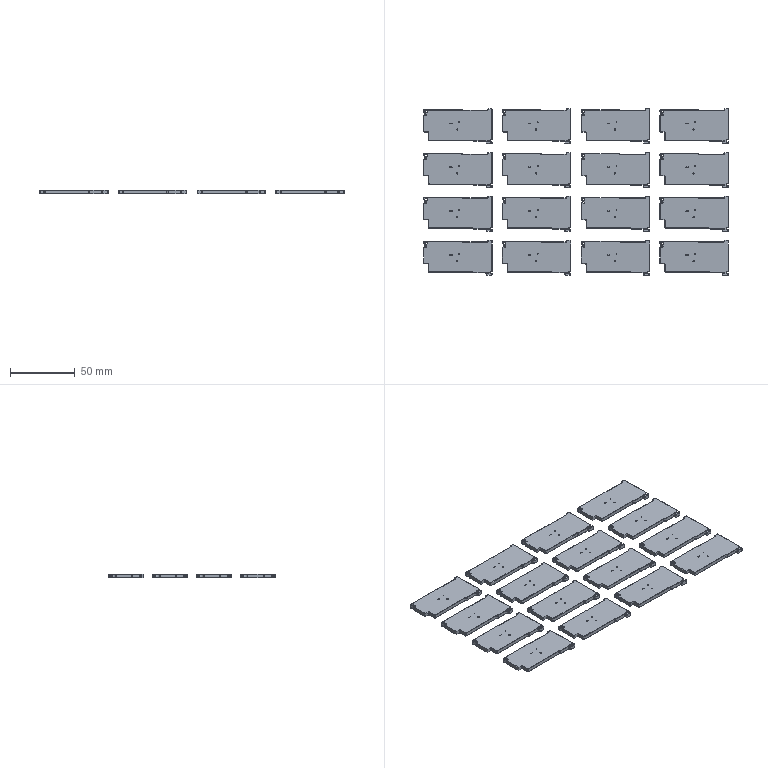NC program | NX | posted with a generic post | part box 236.046 x 129.136 x 3 mm
Whole program:
N10 G17 G21 G94 G90
(DRILLING_COPY , TOOL : D4A45)
N12 T02 M6
N14 G54
N16 G17 G0 G90 X3.25 Y-25.136 S5000 M3
N18 G43 Z30. H2
N20 G94 G81 G98 Z-0.6 F250. R3.
N22 X26.95 Y-16.156
N24 X25.72 Y-10.476
N26 X31.181 Y-11.492
N28 X32.578
N30 X51.15 Y-2.336
N32 X51.058 Y-4.776
N34 G80
N36 G0 X51.058 Y-4.776 Z30.
N38 M5
(DRILLING_COPY_COPY_COPY_COPY_COPY , TOOL : 1.8ZT)
N40 T18 M6
N42 G54
N44 G17 G0 G90 X51.15 Y-2.336 S1910 M3
N46 G43 Z30. H18
N48 G94 G83 G98 Z-5.011 F180. Q2. R3.
N50 G80
N52 G0 X51.15 Y-2.336 Z30.
N54 M5
(DRILLING_COPY_COPY_COPY_COPY_COPY_COPY , TOOL : 1.1ZT)
N56 T13 M6
N58 G54
N60 G17 G0 G90 X3.25 Y-25.136 S2000 M3
N62 G43 Z30. H13
N64 G94 G83 G98 Z-4.8 F100. Q2. R3.
N66 G80
N68 G0 X3.25 Y-25.136 Z30.
N70 M5
(DRILLING_COPY_COPY_COPY_COPY_COPY_COPY_COPY , TOOL : 0.95ZT)
N72 T19 M6
N74 G54
N76 G17 G0 G90 X26.95 Y-16.156 S2122 M3
N78 G43 Z30. H19
N80 G94 G83 G98 Z-4.77 F70. Q2. R3.
N82 G80
N84 G0 X26.95 Y-16.156 Z30.
N86 M5
(DRILLING_COPY_COPY_COPY_COPY_COPY_COPY_COPY_COPY , TOOL : 0.6ZT)
N88 T16 M6
N90 G54
N92 G17 G0 G90 X25.72 Y-10.476 S2000 M3
N94 G43 Z30. H16
N96 G94 G83 G98 Z-4.68 F50. Q0.5 R3.
N98 X31.181 Y-11.492
N100 X32.578
N102 G80
N104 G0 X32.578 Y-11.492 Z30.
N106 M5
(ZLEVEL_PROFILE_COPY_COPY_1_COPY_COPY_1 , TOOL : D0.8)
N108 T20 M6
N110 G54
N112 G17 G0 G90 X50.912 Y-4.864 S9500 M3
N114 G43 Z30. H20
N116 Z1.
N118 G94 G1 X50.959 Y-4.926 Z0.996 F1000.
N120 X51.09 Z0.989
N122 X51.119 Y-4.913 Z0.987
N124 X51.302 Y-4.832 Z0.977
N126 X51.366 Y-4.804 Z0.973
N128 X51.413 Y-4.642 Z0.964
N130 X51.341 Y-4.545 Z0.958
N132 X51.21 Z0.951
N134 X51.181 Y-4.558 Z0.95
N136 X50.998 Y-4.639 Z0.939
N138 X50.934 Y-4.667 Z0.935
N140 X50.887 Y-4.829 Z0.927
N142 X50.959 Y-4.926 Z0.92
N144 X51.09 Z0.913
N146 X51.119 Y-4.913 Z0.912
N148 X51.302 Y-4.832 Z0.901
N150 X51.366 Y-4.804 Z0.898
N152 X51.413 Y-4.642 Z0.889
N154 X51.341 Y-4.545 Z0.882
N156 X51.21 Z0.875
N158 X51.181 Y-4.558 Z0.874
N160 X50.998 Y-4.639 Z0.863
N162 X50.934 Y-4.667 Z0.86
N164 X50.887 Y-4.829 Z0.851
N166 X50.959 Y-4.926 Z0.844
N168 X51.09 Z0.838
N170 X51.119 Y-4.913 Z0.836
N172 X51.302 Y-4.832 Z0.825
N174 X51.366 Y-4.804 Z0.822
N176 X51.413 Y-4.642 Z0.813
N178 X51.341 Y-4.545 Z0.807
N180 X51.21 Z0.8
N182 X51.181 Y-4.558 Z0.798
N184 X50.998 Y-4.639 Z0.788
N186 X50.934 Y-4.667 Z0.784
N188 X50.887 Y-4.829 Z0.775
N190 X50.959 Y-4.926 Z0.769
N192 X51.09 Z0.762
N194 X51.119 Y-4.913 Z0.76
N196 X51.302 Y-4.832 Z0.75
N198 X51.366 Y-4.804 Z0.746
N200 X51.413 Y-4.642 Z0.737
N202 X51.341 Y-4.545 Z0.731
N204 X51.21 Z0.724
N206 X51.181 Y-4.558 Z0.722
N208 X50.998 Y-4.639 Z0.712
N210 X50.934 Y-4.667 Z0.708
N212 X50.887 Y-4.829 Z0.699
N214 X50.959 Y-4.926 Z0.693
N216 X51.09 Z0.686
N218 X51.119 Y-4.913 Z0.685
N220 X51.302 Y-4.832 Z0.674
N222 X51.366 Y-4.804 Z0.67
N224 X51.413 Y-4.642 Z0.662
N226 X51.341 Y-4.545 Z0.655
N228 X51.21 Z0.648
N230 X51.181 Y-4.558 Z0.647
N232 X50.998 Y-4.639 Z0.636
N234 X50.934 Y-4.667 Z0.633
N236 X50.887 Y-4.829 Z0.624
N238 X50.959 Y-4.926 Z0.617
N240 X51.09 Z0.61
N242 X51.119 Y-4.913 Z0.609
N244 X51.302 Y-4.832 Z0.598
N246 X51.366 Y-4.804 Z0.595
N248 X51.413 Y-4.642 Z0.586
N250 X51.341 Y-4.545 Z0.579
N252 X51.21 Z0.573
N254 X51.181 Y-4.558 Z0.571
N256 X50.998 Y-4.639 Z0.56
N258 X50.934 Y-4.667 Z0.557
N260 X50.887 Y-4.829 Z0.548
N262 X50.959 Y-4.926 Z0.542
N264 X51.09 Z0.535
N266 X51.119 Y-4.913 Z0.533
N268 X51.302 Y-4.832 Z0.523
N270 X51.366 Y-4.804 Z0.519
N272 X51.413 Y-4.642 Z0.51
N274 X51.341 Y-4.545 Z0.504
N276 X51.21 Z0.497
N278 X51.181 Y-4.558 Z0.495
N280 X50.998 Y-4.639 Z0.485
N282 X50.934 Y-4.667 Z0.481
N284 X50.887 Y-4.829 Z0.472
N286 X50.959 Y-4.926 Z0.466
N288 X51.09 Z0.459
N290 X51.119 Y-4.913 Z0.457
N292 X51.302 Y-4.832 Z0.447
N294 X51.366 Y-4.804 Z0.443
N296 X51.413 Y-4.642 Z0.434
N298 X51.341 Y-4.545 Z0.428
N300 X51.21 Z0.421
N302 X51.181 Y-4.558 Z0.42
N304 X50.998 Y-4.639 Z0.409
N306 X50.934 Y-4.667 Z0.405
N308 X50.887 Y-4.829 Z0.397
N310 X50.959 Y-4.926 Z0.39
N312 X51.09 Z0.383
N314 X51.119 Y-4.913 Z0.382
N316 X51.302 Y-4.832 Z0.371
N318 X51.366 Y-4.804 Z0.368
N320 X51.413 Y-4.642 Z0.359
N322 X51.341 Y-4.545 Z0.352
N324 X51.21 Z0.345
N326 X51.181 Y-4.558 Z0.344
N328 X50.998 Y-4.639 Z0.333
N330 X50.934 Y-4.667 Z0.33
N332 X50.887 Y-4.829 Z0.321
N334 X50.959 Y-4.926 Z0.314
N336 X51.09 Z0.308
N338 X51.119 Y-4.913 Z0.306
N340 X51.302 Y-4.832 Z0.295
N342 X51.366 Y-4.804 Z0.292
N344 X51.413 Y-4.642 Z0.283
N346 X51.341 Y-4.545 Z0.277
N348 X51.21 Z0.27
N350 X51.181 Y-4.558 Z0.268
N352 X50.998 Y-4.639 Z0.258
N354 X50.934 Y-4.667 Z0.254
N356 X50.887 Y-4.829 Z0.245
N358 X50.959 Y-4.926 Z0.239
N360 X51.09 Z0.232
N362 X51.119 Y-4.913 Z0.23
N364 X51.302 Y-4.832 Z0.22
N366 X51.366 Y-4.804 Z0.216
N368 X51.413 Y-4.642 Z0.207
N370 X51.341 Y-4.545 Z0.201
N372 X51.21 Z0.194
N374 X51.181 Y-4.558 Z0.192
N376 X50.998 Y-4.639 Z0.182
N378 X50.934 Y-4.667 Z0.178
N380 X50.887 Y-4.829 Z0.169
N382 X50.959 Y-4.926 Z0.163
N384 X51.09 Z0.156
N386 X51.119 Y-4.913 Z0.155
N388 X51.302 Y-4.832 Z0.144
N390 X51.366 Y-4.804 Z0.14
N392 X51.413 Y-4.642 Z0.132
N394 X51.341 Y-4.545 Z0.125
N396 X51.21 Z0.118
N398 X51.181 Y-4.558 Z0.117
N400 X50.998 Y-4.639 Z0.106
N402 X50.934 Y-4.667 Z0.103
N404 X50.887 Y-4.829 Z0.094
N406 X50.959 Y-4.926 Z0.087
N408 X51.09 Z0.08
N410 X51.119 Y-4.913 Z0.079
N412 X51.302 Y-4.832 Z0.068
N414 X51.366 Y-4.804 Z0.065
N416 X51.413 Y-4.642 Z0.056
N418 X51.341 Y-4.545 Z0.049
N420 X51.21 Z0.043
N422 X51.181 Y-4.558 Z0.041
N424 X50.998 Y-4.639 Z0.03
N426 X50.934 Y-4.667 Z0.027
N428 X50.887 Y-4.829 Z0.018
N430 X50.959 Y-4.926 Z0.012
N432 X51.09 Z0.005
N434 X51.119 Y-4.913 Z0.003
N436 X51.302 Y-4.832 Z-0.007
N438 X51.366 Y-4.804 Z-0.011
N440 X51.413 Y-4.642 Z-0.02
N442 X51.341 Y-4.545 Z-0.026
N444 X51.21 Z-0.033
N446 X51.181 Y-4.558 Z-0.035
N448 X51.089 Y-4.598 Z-0.04
N450 X50.998 Y-4.639 F850.
N452 G3 X50.921 Y-4.837 R0.15
N454 X51.119 Y-4.913 R0.15
N456 G1 X51.302 Y-4.832
N458 G3 X51.378 Y-4.635 R0.15
N460 X51.181 Y-4.558 R0.15
N462 G1 X51.089 Y-4.598
N464 X50.966 Y-4.667 Z-0.046
N466 X50.95 Y-4.684 Z-0.047
N468 X50.909 Y-4.785 Z-0.051
N470 X50.921 Y-4.837 Z-0.053
N472 X50.98 Y-4.893 Z-0.057
N474 X51.053 Y-4.918 Z-0.06
N476 X51.105 Y-4.91 Z-0.062
N478 X51.21 Y-4.873 Z-0.067
N480 X51.323 Y-4.81 Z-0.072
N482 X51.35 Y-4.787 Z-0.073
N484 X51.382 Y-4.713 Z-0.077
N486 X51.378 Y-4.635 Z-0.08
N488 G3 X51.181 Y-4.558 R0.15
N490 G1 X51.089 Y-4.598
N492 X50.966 Y-4.667 Z-0.086
N494 X50.95 Y-4.684 Z-0.087
N496 X50.909 Y-4.785 Z-0.091
N498 X50.921 Y-4.837 Z-0.093
N500 X50.98 Y-4.893 Z-0.097
N502 X51.053 Y-4.918 Z-0.1
N504 X51.105 Y-4.91 Z-0.102
N506 X51.21 Y-4.873 Z-0.107
N508 X51.323 Y-4.81 Z-0.112
N510 X51.35 Y-4.787 Z-0.113
N512 X51.382 Y-4.713 Z-0.117
N514 X51.378 Y-4.635 Z-0.12
N516 G3 X51.181 Y-4.558 R0.15
N518 G1 X51.089 Y-4.598
N520 X50.966 Y-4.667 Z-0.126
N522 X50.95 Y-4.684 Z-0.127
N524 X50.909 Y-4.785 Z-0.131
N526 X50.921 Y-4.837 Z-0.133
N528 X50.98 Y-4.893 Z-0.137
N530 X51.053 Y-4.918 Z-0.14
N532 X51.105 Y-4.91 Z-0.142
N534 X51.21 Y-4.873 Z-0.147
N536 X51.323 Y-4.81 Z-0.152
N538 X51.35 Y-4.787 Z-0.153
N540 X51.382 Y-4.713 Z-0.157
N542 X51.378 Y-4.635 Z-0.16
N544 G3 X51.181 Y-4.558 R0.15
N546 G1 X51.089 Y-4.598
N548 X50.966 Y-4.667 Z-0.166
N550 X50.95 Y-4.684 Z-0.167
N552 X50.909 Y-4.784 Z-0.171
N554 X50.921 Y-4.837 Z-0.173
N556 X50.98 Y-4.893 Z-0.177
N558 X51.053 Y-4.918 Z-0.18
N560 X51.105 Y-4.91 Z-0.182
N562 X51.21 Y-4.873 Z-0.187
N564 X51.323 Y-4.81 Z-0.192
N566 X51.35 Y-4.787 Z-0.193
N568 X51.382 Y-4.713 Z-0.197
N570 X51.378 Y-4.635 Z-0.2
N572 G3 X51.181 Y-4.558 R0.15
N574 G1 X51.089 Y-4.598
N576 X50.966 Y-4.667 Z-0.206
N578 X50.95 Y-4.684 Z-0.207
N580 X50.909 Y-4.784 Z-0.211
N582 X50.921 Y-4.837 Z-0.213
N584 X50.98 Y-4.893 Z-0.217
N586 X51.053 Y-4.918 Z-0.22
N588 X51.105 Y-4.91 Z-0.222
N590 X51.21 Y-4.873 Z-0.227
N592 X51.323 Y-4.81 Z-0.232
N594 X51.35 Y-4.787 Z-0.233
N596 X51.382 Y-4.713 Z-0.237
N598 X51.378 Y-4.635 Z-0.24
N600 G3 X51.181 Y-4.558 R0.15
N602 G1 X51.089 Y-4.598
N604 X50.966 Y-4.667 Z-0.246
N606 X50.95 Y-4.684 Z-0.247
N608 X50.909 Y-4.784 Z-0.251
N610 X50.921 Y-4.837 Z-0.253
N612 X50.98 Y-4.893 Z-0.257
N614 X51.053 Y-4.918 Z-0.26
N616 X51.105 Y-4.91 Z-0.262
N618 X51.21 Y-4.873 Z-0.267
N620 X51.323 Y-4.81 Z-0.272
N622 X51.35 Y-4.787 Z-0.273
N624 X51.382 Y-4.713 Z-0.277
N626 X51.378 Y-4.635 Z-0.28
N628 G3 X51.181 Y-4.558 R0.15
N630 G1 X51.089 Y-4.598
N632 X50.966 Y-4.667 Z-0.286
N634 X50.95 Y-4.684 Z-0.287
N636 X50.909 Y-4.784 Z-0.291
N638 X50.921 Y-4.837 Z-0.293
N640 X50.98 Y-4.893 Z-0.297
N642 X51.053 Y-4.918 Z-0.3
N644 X51.105 Y-4.91 Z-0.302
N646 X51.21 Y-4.873 Z-0.307
N648 X51.323 Y-4.81 Z-0.312
N650 X51.35 Y-4.787 Z-0.313
N652 X51.382 Y-4.713 Z-0.317
N654 X51.378 Y-4.635 Z-0.32
N656 G3 X51.181 Y-4.558 R0.15
N658 G1 X51.089 Y-4.598
N660 X50.966 Y-4.667 Z-0.326
N662 X50.95 Y-4.684 Z-0.327
N664 X50.909 Y-4.784 Z-0.331
N666 X50.921 Y-4.837 Z-0.333
N668 X50.98 Y-4.893 Z-0.337
N670 X51.053 Y-4.918 Z-0.34
N672 X51.105 Y-4.91 Z-0.342
N674 X51.21 Y-4.873 Z-0.347
N676 X51.323 Y-4.81 Z-0.352
N678 X51.35 Y-4.787 Z-0.353
N680 X51.382 Y-4.713 Z-0.357
N682 X51.378 Y-4.635 Z-0.36
N684 G3 X51.181 Y-4.558 R0.15
N686 G1 X51.089 Y-4.598
N688 X50.966 Y-4.667 Z-0.366
N690 X50.95 Y-4.684 Z-0.367
N692 X50.909 Y-4.784 Z-0.371
N694 X50.921 Y-4.837 Z-0.373
N696 X50.98 Y-4.893 Z-0.377
N698 X51.053 Y-4.918 Z-0.38
N700 X51.105 Y-4.91 Z-0.382
N702 X51.21 Y-4.873 Z-0.387
N704 X51.323 Y-4.81 Z-0.392
N706 X51.35 Y-4.787 Z-0.393
N708 X51.382 Y-4.713 Z-0.397
N710 X51.378 Y-4.635 Z-0.4
N712 G3 X51.181 Y-4.558 R0.15
N714 G1 X51.089 Y-4.598
N716 X50.966 Y-4.667 Z-0.406
N718 X50.95 Y-4.684 Z-0.407
N720 X50.909 Y-4.784 Z-0.411
N722 X50.921 Y-4.837 Z-0.413
N724 X50.98 Y-4.893 Z-0.417
N726 X51.053 Y-4.918 Z-0.42
N728 X51.105 Y-4.91 Z-0.422
N730 X51.21 Y-4.873 Z-0.427
N732 X51.323 Y-4.81 Z-0.432
N734 X51.35 Y-4.787 Z-0.433
N736 X51.382 Y-4.713 Z-0.437
N738 X51.378 Y-4.635 Z-0.44
N740 G3 X51.181 Y-4.558 R0.15
N742 G1 X51.089 Y-4.598
N744 X50.966 Y-4.667 Z-0.446
N746 X50.95 Y-4.684 Z-0.447
N748 X50.909 Y-4.784 Z-0.451
N750 X50.921 Y-4.837 Z-0.453
N752 X50.98 Y-4.893 Z-0.457
N754 X51.053 Y-4.918 Z-0.46
N756 X51.105 Y-4.91 Z-0.462
N758 X51.21 Y-4.873 Z-0.467
N760 X51.323 Y-4.81 Z-0.472
N762 X51.35 Y-4.787 Z-0.473
N764 X51.382 Y-4.713 Z-0.477
N766 X51.378 Y-4.635 Z-0.48
N768 G3 X51.181 Y-4.558 R0.15
N770 G1 X51.089 Y-4.598
N772 X50.966 Y-4.667 Z-0.486
N774 X50.95 Y-4.684 Z-0.487
N776 X50.909 Y-4.784 Z-0.491
N778 X50.921 Y-4.837 Z-0.493
N780 X50.98 Y-4.893 Z-0.497
N782 X51.053 Y-4.918 Z-0.5
N784 X51.105 Y-4.91 Z-0.502
N786 X51.21 Y-4.873 Z-0.507
N788 X51.323 Y-4.81 Z-0.512
N790 X51.35 Y-4.787 Z-0.513
N792 X51.382 Y-4.713 Z-0.517
N794 X51.378 Y-4.635 Z-0.52
N796 G3 X51.181 Y-4.558 R0.15
N798 G1 X51.089 Y-4.598
N800 X50.966 Y-4.667 Z-0.526
N802 X50.95 Y-4.684 Z-0.527
N804 X50.909 Y-4.784 Z-0.531
N806 X50.921 Y-4.837 Z-0.533
N808 X50.98 Y-4.893 Z-0.537
N810 X51.053 Y-4.918 Z-0.54
N812 X51.105 Y-4.91 Z-0.542
N814 X51.21 Y-4.873 Z-0.547
N816 X51.323 Y-4.81 Z-0.552
N818 X51.35 Y-4.787 Z-0.553
N820 X51.382 Y-4.713 Z-0.557
N822 X51.378 Y-4.635 Z-0.56
N824 G3 X51.181 Y-4.558 R0.15
N826 G1 X51.089 Y-4.598
N828 X50.966 Y-4.667 Z-0.566
N830 X50.95 Y-4.684 Z-0.567
N832 X50.909 Y-4.784 Z-0.571
N834 X50.921 Y-4.837 Z-0.573
N836 X50.98 Y-4.893 Z-0.577
N838 X51.053 Y-4.918 Z-0.58
N840 X51.105 Y-4.91 Z-0.582
N842 X51.21 Y-4.873 Z-0.587
N844 X51.323 Y-4.81 Z-0.592
N846 X51.35 Y-4.787 Z-0.593
N848 X51.382 Y-4.713 Z-0.597
N850 X51.378 Y-4.635 Z-0.6
N852 G3 X51.181 Y-4.558 R0.15
N854 G1 X51.089 Y-4.598
N856 X50.966 Y-4.667 Z-0.606
N858 X50.95 Y-4.684 Z-0.607
N860 X50.909 Y-4.784 Z-0.611
N862 X50.921 Y-4.837 Z-0.613
N864 X50.98 Y-4.893 Z-0.617
N866 X51.053 Y-4.918 Z-0.62
N868 X51.105 Y-4.91 Z-0.622
N870 X51.21 Y-4.873 Z-0.627
N872 X51.323 Y-4.81 Z-0.632
N874 X51.35 Y-4.787 Z-0.633
N876 X51.382 Y-4.713 Z-0.637
N878 X51.378 Y-4.635 Z-0.64
N880 G3 X51.181 Y-4.558 R0.15
N882 G1 X51.089 Y-4.598
N884 X50.966 Y-4.667 Z-0.646
N886 X50.95 Y-4.684 Z-0.647
N888 X50.909 Y-4.784 Z-0.651
N890 X50.921 Y-4.837 Z-0.653
N892 X50.98 Y-4.893 Z-0.657
N894 X51.053 Y-4.918 Z-0.66
N896 X51.105 Y-4.91 Z-0.662
N898 X51.21 Y-4.873 Z-0.667
N900 X51.323 Y-4.81 Z-0.672
N902 X51.35 Y-4.787 Z-0.673
N904 X51.382 Y-4.713 Z-0.677
N906 X51.378 Y-4.635 Z-0.68
N908 G3 X51.181 Y-4.558 R0.15
N910 G1 X51.089 Y-4.598
N912 X50.966 Y-4.667 Z-0.686
N914 X50.95 Y-4.684 Z-0.687
N916 X50.909 Y-4.784 Z-0.691
N918 X50.921 Y-4.837 Z-0.693
N920 X50.98 Y-4.893 Z-0.697
N922 X51.053 Y-4.918 Z-0.7
N924 X51.105 Y-4.91 Z-0.702
N926 X51.21 Y-4.873 Z-0.707
N928 X51.323 Y-4.81 Z-0.712
N930 X51.35 Y-4.787 Z-0.713
N932 X51.382 Y-4.713 Z-0.717
N934 X51.378 Y-4.635 Z-0.72
N936 G3 X51.181 Y-4.558 R0.15
N938 G1 X51.089 Y-4.598
N940 X50.966 Y-4.667 Z-0.726
N942 X50.95 Y-4.684 Z-0.727
N944 X50.909 Y-4.784 Z-0.731
N946 X50.921 Y-4.837 Z-0.733
N948 X50.98 Y-4.893 Z-0.737
N950 X51.053 Y-4.918 Z-0.74
N952 X51.105 Y-4.91 Z-0.742
N954 X51.21 Y-4.873 Z-0.747
N956 X51.323 Y-4.81 Z-0.752
N958 X51.35 Y-4.787 Z-0.753
N960 X51.382 Y-4.713 Z-0.757
N962 X51.378 Y-4.635 Z-0.76
N964 G3 X51.181 Y-4.558 R0.15
N966 G1 X51.089 Y-4.598
N968 X50.966 Y-4.667 Z-0.766
N970 X50.95 Y-4.684 Z-0.767
N972 X50.909 Y-4.784 Z-0.771
N974 X50.921 Y-4.837 Z-0.773
N976 X50.98 Y-4.893 Z-0.777
N978 X51.053 Y-4.918 Z-0.78
N980 X51.105 Y-4.91 Z-0.782
N982 X51.21 Y-4.873 Z-0.787
N984 X51.323 Y-4.81 Z-0.792
N986 X51.35 Y-4.787 Z-0.793
N988 X51.382 Y-4.713 Z-0.797
N990 X51.378 Y-4.635 Z-0.8
N992 G3 X51.181 Y-4.558 R0.15
N994 G1 X51.089 Y-4.598
N996 X50.966 Y-4.667 Z-0.806
N998 X50.95 Y-4.684 Z-0.807
N1000 X50.909 Y-4.784 Z-0.811
N1002 X50.921 Y-4.837 Z-0.813
N1004 X50.98 Y-4.893 Z-0.817
N1006 X51.053 Y-4.918 Z-0.82
N1008 X51.105 Y-4.91 Z-0.822
N1010 X51.21 Y-4.873 Z-0.827
N1012 X51.323 Y-4.81 Z-0.832
N1014 X51.35 Y-4.787 Z-0.833
N1016 X51.382 Y-4.713 Z-0.837
N1018 X51.378 Y-4.635 Z-0.84
N1020 G3 X51.181 Y-4.558 R0.15
N1022 G1 X51.089 Y-4.598
N1024 X50.966 Y-4.667 Z-0.846
N1026 X50.95 Y-4.684 Z-0.847
N1028 X50.909 Y-4.784 Z-0.851
N1030 X50.921 Y-4.837 Z-0.853
N1032 X50.98 Y-4.893 Z-0.857
N1034 X51.053 Y-4.918 Z-0.86
N1036 X51.105 Y-4.91 Z-0.862
N1038 X51.21 Y-4.873 Z-0.867
N1040 X51.323 Y-4.81 Z-0.872
N1042 X51.35 Y-4.787 Z-0.873
N1044 X51.382 Y-4.713 Z-0.877
N1046 X51.378 Y-4.635 Z-0.88
N1048 G3 X51.181 Y-4.558 R0.15
N1050 G1 X51.089 Y-4.598
N1052 X50.966 Y-4.667 Z-0.886
N1054 X50.95 Y-4.684 Z-0.887
N1056 X50.909 Y-4.784 Z-0.891
N1058 X50.921 Y-4.837 Z-0.893
N1060 X50.98 Y-4.893 Z-0.897
N1062 X51.053 Y-4.918 Z-0.9
N1064 X51.105 Y-4.91 Z-0.902
N1066 X51.21 Y-4.873 Z-0.907
N1068 X51.323 Y-4.81 Z-0.912
N1070 X51.35 Y-4.787 Z-0.913
N1072 X51.382 Y-4.713 Z-0.917
N1074 X51.378 Y-4.635 Z-0.92
N1076 G3 X51.181 Y-4.558 R0.15
N1078 G1 X51.089 Y-4.598
N1080 X50.966 Y-4.667 Z-0.926
N1082 X50.95 Y-4.684 Z-0.927
N1084 X50.909 Y-4.784 Z-0.931
N1086 X50.921 Y-4.837 Z-0.933
N1088 X50.98 Y-4.893 Z-0.937
N1090 X51.053 Y-4.918 Z-0.94
N1092 X51.105 Y-4.91 Z-0.942
N1094 X51.21 Y-4.873 Z-0.947
N1096 X51.323 Y-4.81 Z-0.952
N1098 X51.35 Y-4.787 Z-0.953
N1100 X51.382 Y-4.713 Z-0.957
N1102 X51.378 Y-4.635 Z-0.96
N1104 G3 X51.181 Y-4.558 R0.15
N1106 G1 X51.089 Y-4.598
N1108 X50.966 Y-4.667 Z-0.966
N1110 X50.95 Y-4.684 Z-0.967
N1112 X50.909 Y-4.784 Z-0.971
N1114 X50.921 Y-4.837 Z-0.973
N1116 X50.98 Y-4.893 Z-0.977
N1118 X51.053 Y-4.918 Z-0.98
N1120 X51.105 Y-4.91 Z-0.982
N1122 X51.21 Y-4.873 Z-0.987
N1124 X51.323 Y-4.81 Z-0.992
N1126 X51.35 Y-4.787 Z-0.993
N1128 X51.382 Y-4.713 Z-0.997
N1130 X51.378 Y-4.635 Z-1.
N1132 G3 X51.181 Y-4.558 R0.15
N1134 G1 X51.089 Y-4.598
N1136 X50.966 Y-4.667 Z-1.006
N1138 X50.95 Y-4.684 Z-1.007
N1140 X50.909 Y-4.784 Z-1.011
N1142 X50.921 Y-4.837 Z-1.013
N1144 X50.98 Y-4.893 Z-1.017
N1146 X51.053 Y-4.918 Z-1.02
N1148 X51.105 Y-4.91 Z-1.022
N1150 X51.21 Y-4.873 Z-1.027
N1152 X51.323 Y-4.81 Z-1.032
N1154 X51.35 Y-4.787 Z-1.033
N1156 X51.382 Y-4.713 Z-1.037
N1158 X51.378 Y-4.635 Z-1.04
N1160 G3 X51.181 Y-4.558 R0.15
N1162 G1 X51.089 Y-4.598
N1164 X50.966 Y-4.667 Z-1.046
N1166 X50.95 Y-4.684 Z-1.047
N1168 X50.909 Y-4.784 Z-1.051
N1170 X50.921 Y-4.837 Z-1.053
N1172 X50.98 Y-4.893 Z-1.057
N1174 X51.053 Y-4.918 Z-1.06
N1176 X51.105 Y-4.91 Z-1.062
N1178 X51.21 Y-4.873 Z-1.067
N1180 X51.323 Y-4.81 Z-1.072
N1182 X51.35 Y-4.787 Z-1.073
N1184 X51.382 Y-4.713 Z-1.077
N1186 X51.378 Y-4.635 Z-1.08
N1188 G3 X51.181 Y-4.558 R0.15
N1190 G1 X51.089 Y-4.598
N1192 X50.966 Y-4.667 Z-1.086
N1194 X50.95 Y-4.684 Z-1.087
N1196 X50.909 Y-4.784 Z-1.091
N1198 X50.921 Y-4.837 Z-1.093
N1200 X50.98 Y-4.893 Z-1.097
N1202 X51.053 Y-4.918 Z-1.1
N1204 X51.105 Y-4.91 Z-1.102
N1206 X51.21 Y-4.873 Z-1.107
N1208 X51.323 Y-4.81 Z-1.112
N1210 X51.35 Y-4.787 Z-1.113
N1212 X51.382 Y-4.713 Z-1.117
N1214 X51.378 Y-4.635 Z-1.12
N1216 G3 X51.181 Y-4.558 R0.15
N1218 G1 X51.089 Y-4.598
N1220 X50.966 Y-4.667 Z-1.126
N1222 X50.95 Y-4.684 Z-1.127
N1224 X50.909 Y-4.784 Z-1.131
N1226 X50.921 Y-4.837 Z-1.133
N1228 X50.98 Y-4.893 Z-1.137
N1230 X51.053 Y-4.918 Z-1.14
N1232 X51.105 Y-4.91 Z-1.142
N1234 X51.21 Y-4.873 Z-1.147
N1236 X51.323 Y-4.81 Z-1.152
N1238 X51.35 Y-4.787 Z-1.153
N1240 X51.382 Y-4.713 Z-1.157
N1242 X51.378 Y-4.635 Z-1.16
N1244 G3 X51.181 Y-4.558 R0.15
N1246 G1 X51.089 Y-4.598
N1248 X50.966 Y-4.667 Z-1.166
N1250 X50.95 Y-4.684 Z-1.167
N1252 X50.909 Y-4.784 Z-1.171
N1254 X50.921 Y-4.837 Z-1.173
N1256 X50.98 Y-4.893 Z-1.177
N1258 X51.053 Y-4.918 Z-1.18
N1260 X51.105 Y-4.91 Z-1.182
N1262 X51.21 Y-4.873 Z-1.187
N1264 X51.323 Y-4.81 Z-1.192
N1266 X51.35 Y-4.787 Z-1.193
N1268 X51.382 Y-4.713 Z-1.197
N1270 X51.378 Y-4.635 Z-1.2
N1272 G3 X51.181 Y-4.558 R0.15
N1274 G1 X51.089 Y-4.598
N1276 X50.966 Y-4.667 Z-1.206
N1278 X50.95 Y-4.684 Z-1.207
N1280 X50.909 Y-4.784 Z-1.211
N1282 X50.921 Y-4.837 Z-1.213
N1284 X50.98 Y-4.893 Z-1.217
N1286 X51.053 Y-4.918 Z-1.22
N1288 X51.105 Y-4.91 Z-1.222
N1290 X51.21 Y-4.873 Z-1.227
N1292 X51.323 Y-4.81 Z-1.232
N1294 X51.35 Y-4.787 Z-1.233
N1296 X51.382 Y-4.713 Z-1.237
N1298 X51.378 Y-4.635 Z-1.24
N1300 G3 X51.181 Y-4.558 R0.15
N1302 G1 X51.089 Y-4.598
N1304 X50.966 Y-4.667 Z-1.246
N1306 X50.95 Y-4.684 Z-1.247
N1308 X50.909 Y-4.784 Z-1.251
N1310 X50.921 Y-4.837 Z-1.253
N1312 X50.98 Y-4.893 Z-1.257
N1314 X51.053 Y-4.918 Z-1.26
N1316 X51.105 Y-4.91 Z-1.262
N1318 X51.21 Y-4.873 Z-1.267
N1320 X51.323 Y-4.81 Z-1.272
N1322 X51.35 Y-4.787 Z-1.273
N1324 X51.382 Y-4.713 Z-1.277
N1326 X51.378 Y-4.635 Z-1.28
N1328 G3 X51.181 Y-4.558 R0.15
N1330 G1 X51.089 Y-4.598
N1332 X50.966 Y-4.667 Z-1.286
N1334 X50.95 Y-4.684 Z-1.287
N1336 X50.909 Y-4.784 Z-1.291
N1338 X50.921 Y-4.837 Z-1.293
N1340 X50.98 Y-4.893 Z-1.297
N1342 X51.053 Y-4.918 Z-1.3
N1344 X51.105 Y-4.91 Z-1.302
N1346 X51.21 Y-4.873 Z-1.307
N1348 X51.323 Y-4.81 Z-1.312
N1350 X51.35 Y-4.787 Z-1.313
N1352 X51.382 Y-4.713 Z-1.317
N1354 X51.378 Y-4.635 Z-1.32
N1356 G3 X51.181 Y-4.558 R0.15
N1358 G1 X51.089 Y-4.598
N1360 X50.966 Y-4.667 Z-1.326
N1362 X50.95 Y-4.684 Z-1.327
N1364 X50.909 Y-4.784 Z-1.331
N1366 X50.921 Y-4.837 Z-1.333
N1368 X50.98 Y-4.893 Z-1.337
N1370 X51.053 Y-4.918 Z-1.34
N1372 X51.105 Y-4.91 Z-1.342
N1374 X51.21 Y-4.873 Z-1.347
N1376 X51.323 Y-4.81 Z-1.352
N1378 X51.35 Y-4.787 Z-1.353
N1380 X51.382 Y-4.713 Z-1.357
N1382 X51.378 Y-4.635 Z-1.36
N1384 G3 X51.181 Y-4.558 R0.15
N1386 G1 X51.089 Y-4.598
N1388 X50.966 Y-4.667 Z-1.366
N1390 X50.95 Y-4.684 Z-1.367
N1392 X50.909 Y-4.784 Z-1.371
N1394 X50.921 Y-4.837 Z-1.373
N1396 X50.98 Y-4.893 Z-1.377
N1398 X51.053 Y-4.918 Z-1.38
N1400 X51.105 Y-4.91 Z-1.382
N1402 X51.21 Y-4.873 Z-1.387
N1404 X51.323 Y-4.81 Z-1.392
N1406 X51.35 Y-4.787 Z-1.393
N1408 X51.382 Y-4.713 Z-1.397
N1410 X51.378 Y-4.635 Z-1.4
N1412 G3 X51.181 Y-4.558 R0.15
N1414 G1 X51.089 Y-4.598
N1416 X50.966 Y-4.667 Z-1.406
N1418 X50.95 Y-4.684 Z-1.407
N1420 X50.909 Y-4.784 Z-1.411
N1422 X50.921 Y-4.837 Z-1.413
N1424 X50.98 Y-4.893 Z-1.417
N1426 X51.053 Y-4.918 Z-1.42
N1428 X51.105 Y-4.91 Z-1.422
N1430 X51.21 Y-4.873 Z-1.427
N1432 X51.323 Y-4.81 Z-1.432
N1434 X51.35 Y-4.787 Z-1.433
N1436 X51.382 Y-4.713 Z-1.437
N1438 X51.378 Y-4.635 Z-1.44
N1440 G3 X51.181 Y-4.558 R0.15
N1442 G1 X51.089 Y-4.598
N1444 X50.966 Y-4.667 Z-1.446
N1446 X50.95 Y-4.684 Z-1.447
N1448 X50.909 Y-4.784 Z-1.451
N1450 X50.921 Y-4.837 Z-1.453
N1452 X50.98 Y-4.893 Z-1.457
N1454 X51.053 Y-4.918 Z-1.46
N1456 X51.105 Y-4.91 Z-1.462
N1458 X51.21 Y-4.873 Z-1.467
N1460 X51.323 Y-4.81 Z-1.472
N1462 X51.35 Y-4.787 Z-1.473
N1464 X51.382 Y-4.713 Z-1.477
N1466 X51.378 Y-4.635 Z-1.48
N1468 G3 X51.181 Y-4.558 R0.15
N1470 G1 X51.089 Y-4.598
N1472 X50.966 Y-4.667 Z-1.486
N1474 X50.95 Y-4.684 Z-1.487
N1476 X50.909 Y-4.784 Z-1.491
N1478 X50.921 Y-4.837 Z-1.493
N1480 X50.98 Y-4.893 Z-1.497
N1482 X51.053 Y-4.918 Z-1.5
N1484 X51.105 Y-4.91 Z-1.502
N1486 X51.21 Y-4.873 Z-1.507
N1488 X51.323 Y-4.81 Z-1.512
N1490 X51.35 Y-4.787 Z-1.513
N1492 X51.382 Y-4.713 Z-1.517
N1494 X51.378 Y-4.635 Z-1.52
N1496 G3 X51.181 Y-4.558 R0.15
N1498 G1 X51.089 Y-4.598
N1500 X50.966 Y-4.667 Z-1.526
N1502 X50.95 Y-4.684 Z-1.527
N1504 X50.909 Y-4.784 Z-1.531
N1506 X50.921 Y-4.837 Z-1.533
N1508 X50.98 Y-4.893 Z-1.537
N1510 X51.053 Y-4.918 Z-1.54
N1512 X51.105 Y-4.91 Z-1.542
N1514 X51.21 Y-4.873 Z-1.547
N1516 X51.323 Y-4.81 Z-1.552
N1518 X51.35 Y-4.787 Z-1.553
N1520 X51.382 Y-4.713 Z-1.557
N1522 X51.378 Y-4.635 Z-1.56
N1524 G3 X51.181 Y-4.558 R0.15
N1526 G1 X51.089 Y-4.598
N1528 X50.966 Y-4.667 Z-1.566
N1530 X50.95 Y-4.684 Z-1.567
N1532 X50.909 Y-4.784 Z-1.571
N1534 X50.921 Y-4.837 Z-1.573
N1536 X50.98 Y-4.893 Z-1.577
N1538 X51.053 Y-4.918 Z-1.58
N1540 X51.105 Y-4.91 Z-1.582
N1542 X51.21 Y-4.873 Z-1.587
N1544 X51.323 Y-4.81 Z-1.592
N1546 X51.35 Y-4.787 Z-1.593
N1548 X51.382 Y-4.713 Z-1.597
N1550 X51.378 Y-4.635 Z-1.6
N1552 G3 X51.181 Y-4.558 R0.15
N1554 G1 X51.089 Y-4.598
N1556 X50.966 Y-4.667 Z-1.606
N1558 X50.95 Y-4.684 Z-1.607
N1560 X50.909 Y-4.784 Z-1.611
N1562 X50.921 Y-4.837 Z-1.613
N1564 X50.98 Y-4.893 Z-1.617
N1566 X51.053 Y-4.918 Z-1.62
N1568 X51.105 Y-4.91 Z-1.622
N1570 X51.21 Y-4.873 Z-1.627
N1572 X51.323 Y-4.81 Z-1.632
N1574 X51.35 Y-4.787 Z-1.633
N1576 X51.382 Y-4.713 Z-1.637
N1578 X51.378 Y-4.635 Z-1.64
N1580 G3 X51.181 Y-4.558 R0.15
N1582 G1 X51.089 Y-4.598
N1584 X50.966 Y-4.667 Z-1.646
N1586 X50.95 Y-4.684 Z-1.647
N1588 X50.909 Y-4.784 Z-1.651
N1590 X50.921 Y-4.837 Z-1.653
N1592 X50.98 Y-4.893 Z-1.657
N1594 X51.053 Y-4.918 Z-1.66
N1596 X51.105 Y-4.91 Z-1.662
N1598 X51.21 Y-4.873 Z-1.667
N1600 X51.323 Y-4.81 Z-1.672
N1602 X51.35 Y-4.787 Z-1.673
N1604 X51.382 Y-4.713 Z-1.677
N1606 X51.378 Y-4.635 Z-1.68
N1608 G3 X51.181 Y-4.558 R0.15
N1610 G1 X51.089 Y-4.598
N1612 X50.966 Y-4.667 Z-1.686
N1614 X50.95 Y-4.684 Z-1.687
N1616 X50.909 Y-4.784 Z-1.691
N1618 X50.921 Y-4.837 Z-1.693
N1620 X50.98 Y-4.893 Z-1.697
N1622 X51.053 Y-4.918 Z-1.7
N1624 X51.105 Y-4.91 Z-1.702
N1626 X51.21 Y-4.873 Z-1.707
N1628 X51.323 Y-4.81 Z-1.712
N1630 X51.35 Y-4.787 Z-1.713
N1632 X51.382 Y-4.713 Z-1.717
N1634 X51.378 Y-4.635 Z-1.72
N1636 G3 X51.181 Y-4.558 R0.15
N1638 G1 X51.089 Y-4.598
N1640 X50.966 Y-4.667 Z-1.726
N1642 X50.95 Y-4.684 Z-1.727
N1644 X50.909 Y-4.784 Z-1.731
N1646 X50.921 Y-4.837 Z-1.733
N1648 X50.98 Y-4.893 Z-1.737
N1650 X51.053 Y-4.918 Z-1.74
N1652 X51.105 Y-4.91 Z-1.742
N1654 X51.21 Y-4.873 Z-1.747
N1656 X51.323 Y-4.81 Z-1.752
N1658 X51.35 Y-4.787 Z-1.753
N1660 X51.382 Y-4.713 Z-1.757
N1662 X51.378 Y-4.635 Z-1.76
N1664 G3 X51.181 Y-4.558 R0.15
N1666 G1 X51.089 Y-4.598
N1668 X50.966 Y-4.667 Z-1.766
N1670 X50.95 Y-4.684 Z-1.767
N1672 X50.909 Y-4.784 Z-1.771
N1674 X50.921 Y-4.837 Z-1.773
N1676 X50.98 Y-4.893 Z-1.777
N1678 X51.053 Y-4.918 Z-1.78
N1680 X51.105 Y-4.91 Z-1.782
N1682 X51.21 Y-4.873 Z-1.787
N1684 X51.323 Y-4.81 Z-1.792
N1686 X51.35 Y-4.787 Z-1.793
N1688 X51.382 Y-4.713 Z-1.797
N1690 X51.378 Y-4.635 Z-1.8
N1692 G3 X51.181 Y-4.558 R0.15
N1694 G1 X51.089 Y-4.598
N1696 X50.966 Y-4.667 Z-1.806
N1698 X50.95 Y-4.684 Z-1.807
N1700 X50.909 Y-4.784 Z-1.811
N1702 X50.921 Y-4.837 Z-1.813
N1704 X50.98 Y-4.893 Z-1.817
N1706 X51.053 Y-4.918 Z-1.82
N1708 X51.105 Y-4.91 Z-1.822
N1710 X51.21 Y-4.873 Z-1.827
N1712 X51.323 Y-4.81 Z-1.832
N1714 X51.35 Y-4.787 Z-1.833
N1716 X51.382 Y-4.713 Z-1.837
N1718 X51.378 Y-4.635 Z-1.84
N1720 G3 X51.181 Y-4.558 R0.15
N1722 G1 X51.089 Y-4.598
N1724 X50.966 Y-4.667 Z-1.846
N1726 X50.95 Y-4.684 Z-1.847
N1728 X50.909 Y-4.784 Z-1.851
N1730 X50.921 Y-4.837 Z-1.853
N1732 X50.98 Y-4.893 Z-1.857
N1734 X51.053 Y-4.918 Z-1.86
N1736 X51.105 Y-4.91 Z-1.862
N1738 X51.21 Y-4.873 Z-1.867
N1740 X51.323 Y-4.81 Z-1.872
N1742 X51.35 Y-4.787 Z-1.873
N1744 X51.382 Y-4.713 Z-1.877
N1746 X51.378 Y-4.635 Z-1.88
N1748 G3 X51.181 Y-4.558 R0.15
N1750 G1 X51.089 Y-4.598
N1752 X50.966 Y-4.667 Z-1.886
N1754 X50.95 Y-4.684 Z-1.887
N1756 X50.909 Y-4.784 Z-1.891
N1758 X50.921 Y-4.837 Z-1.893
N1760 X50.98 Y-4.893 Z-1.897
N1762 X51.053 Y-4.918 Z-1.9
N1764 X51.105 Y-4.91 Z-1.902
N1766 X51.21 Y-4.873 Z-1.907
N1768 X51.323 Y-4.81 Z-1.912
N1770 X51.35 Y-4.787 Z-1.913
N1772 X51.382 Y-4.713 Z-1.917
N1774 X51.378 Y-4.635 Z-1.92
N1776 G3 X51.181 Y-4.558 R0.15
N1778 G1 X51.089 Y-4.598
N1780 X50.966 Y-4.667 Z-1.926
N1782 X50.95 Y-4.684 Z-1.927
N1784 X50.909 Y-4.784 Z-1.931
N1786 X50.921 Y-4.837 Z-1.933
N1788 X50.98 Y-4.893 Z-1.937
N1790 X51.053 Y-4.918 Z-1.94
N1792 X51.105 Y-4.91 Z-1.942
N1794 X51.21 Y-4.873 Z-1.947
N1796 X51.323 Y-4.81 Z-1.952
N1798 X51.35 Y-4.787 Z-1.953
N1800 X51.382 Y-4.713 Z-1.957
N1802 X51.378 Y-4.635 Z-1.96
N1804 G3 X51.181 Y-4.558 R0.15
N1806 G1 X51.089 Y-4.598
N1808 X50.966 Y-4.667 Z-1.966
N1810 X50.95 Y-4.684 Z-1.967
N1812 X50.909 Y-4.784 Z-1.971
N1814 X50.921 Y-4.837 Z-1.973
N1816 X50.98 Y-4.893 Z-1.977
N1818 X51.053 Y-4.918 Z-1.98
N1820 X51.105 Y-4.91 Z-1.982
N1822 X51.21 Y-4.873 Z-1.987
N1824 X51.323 Y-4.81 Z-1.992
N1826 X51.35 Y-4.787 Z-1.993
N1828 X51.382 Y-4.713 Z-1.997
N1830 X51.378 Y-4.635 Z-2.
N1832 G3 X51.181 Y-4.558 R0.15
N1834 G1 X51.089 Y-4.598
N1836 X50.966 Y-4.667 Z-2.006
N1838 X50.95 Y-4.684 Z-2.007
N1840 X50.909 Y-4.784 Z-2.011
N1842 X50.921 Y-4.837 Z-2.013
N1844 X50.98 Y-4.893 Z-2.017
N1846 X51.053 Y-4.918 Z-2.02
N1848 X51.105 Y-4.91 Z-2.022
N1850 X51.21 Y-4.873 Z-2.027
N1852 X51.323 Y-4.81 Z-2.032
N1854 X51.35 Y-4.787 Z-2.033
N1856 X51.382 Y-4.713 Z-2.037
N1858 X51.378 Y-4.635 Z-2.04
N1860 G3 X51.181 Y-4.558 R0.15
N1862 G1 X51.089 Y-4.598
N1864 X50.966 Y-4.667 Z-2.046
N1866 X50.95 Y-4.684 Z-2.047
N1868 X50.909 Y-4.784 Z-2.051
N1870 X50.921 Y-4.837 Z-2.053
N1872 X50.98 Y-4.893 Z-2.057
N1874 X51.053 Y-4.918 Z-2.06
N1876 X51.105 Y-4.91 Z-2.062
N1878 X51.21 Y-4.873 Z-2.067
N1880 X51.323 Y-4.81 Z-2.072
N1882 X51.35 Y-4.787 Z-2.073
N1884 X51.382 Y-4.713 Z-2.077
N1886 X51.378 Y-4.635 Z-2.08
N1888 G3 X51.181 Y-4.558 R0.15
N1890 G1 X51.089 Y-4.598
N1892 X50.966 Y-4.667 Z-2.086
N1894 X50.95 Y-4.684 Z-2.087
N1896 X50.909 Y-4.784 Z-2.091
N1898 X50.921 Y-4.837 Z-2.093
N1900 X50.98 Y-4.893 Z-2.097
N1902 X51.053 Y-4.918 Z-2.1
N1904 X51.105 Y-4.91 Z-2.102
N1906 X51.21 Y-4.873 Z-2.107
N1908 X51.323 Y-4.81 Z-2.112
N1910 X51.35 Y-4.787 Z-2.113
N1912 X51.382 Y-4.713 Z-2.117
N1914 X51.378 Y-4.635 Z-2.12
N1916 G3 X51.181 Y-4.558 R0.15
N1918 G1 X51.089 Y-4.598
N1920 X50.966 Y-4.667 Z-2.126
N1922 X50.95 Y-4.684 Z-2.127
N1924 X50.909 Y-4.784 Z-2.131
N1926 X50.921 Y-4.837 Z-2.133
N1928 X50.98 Y-4.893 Z-2.137
N1930 X51.053 Y-4.918 Z-2.14
N1932 X51.105 Y-4.91 Z-2.142
N1934 X51.21 Y-4.873 Z-2.147
N1936 X51.323 Y-4.81 Z-2.152
N1938 X51.35 Y-4.787 Z-2.153
N1940 X51.382 Y-4.713 Z-2.157
N1942 X51.378 Y-4.635 Z-2.16
N1944 G3 X51.181 Y-4.558 R0.15
N1946 G1 X51.089 Y-4.598
N1948 X50.966 Y-4.667 Z-2.166
N1950 X50.95 Y-4.684 Z-2.167
N1952 X50.909 Y-4.784 Z-2.171
N1954 X50.921 Y-4.837 Z-2.173
N1956 X50.98 Y-4.893 Z-2.177
N1958 X51.053 Y-4.918 Z-2.18
N1960 X51.105 Y-4.91 Z-2.182
N1962 X51.21 Y-4.873 Z-2.187
N1964 X51.323 Y-4.81 Z-2.192
N1966 X51.35 Y-4.787 Z-2.193
N1968 X51.382 Y-4.713 Z-2.197
N1970 X51.378 Y-4.635 Z-2.2
N1972 G3 X51.181 Y-4.558 R0.15
N1974 G1 X51.089 Y-4.598
N1976 X50.967 Y-4.667 Z-2.206
N1978 X50.95 Y-4.684 Z-2.207
N1980 X50.909 Y-4.784 Z-2.211
N1982 X50.921 Y-4.837 Z-2.213
N1984 X50.98 Y-4.893 Z-2.217
N1986 X51.053 Y-4.918 Z-2.22
N1988 X51.105 Y-4.91 Z-2.222
N1990 X51.21 Y-4.873 Z-2.227
N1992 X51.323 Y-4.81 Z-2.232
N1994 X51.35 Y-4.787 Z-2.233
N1996 X51.382 Y-4.713 Z-2.237
N1998 X51.378 Y-4.635 Z-2.24
N2000 G3 X51.181 Y-4.558 R0.15
N2002 G1 X51.089 Y-4.598
N2004 X50.967 Y-4.667 Z-2.246
N2006 X50.95 Y-4.684 Z-2.247
N2008 X50.909 Y-4.784 Z-2.251
N2010 X50.921 Y-4.837 Z-2.253
N2012 X50.98 Y-4.893 Z-2.257
N2014 X51.053 Y-4.918 Z-2.26
N2016 X51.105 Y-4.91 Z-2.262
N2018 X51.21 Y-4.873 Z-2.267
N2020 X51.323 Y-4.81 Z-2.272
N2022 X51.35 Y-4.787 Z-2.273
N2024 X51.382 Y-4.713 Z-2.277
N2026 X51.378 Y-4.635 Z-2.28
N2028 G3 X51.181 Y-4.558 R0.15
N2030 G1 X51.089 Y-4.598
N2032 X50.967 Y-4.667 Z-2.286
N2034 X50.95 Y-4.684 Z-2.287
N2036 X50.909 Y-4.784 Z-2.291
N2038 X50.921 Y-4.837 Z-2.293
N2040 X50.98 Y-4.893 Z-2.297
N2042 X51.053 Y-4.918 Z-2.3
N2044 X51.105 Y-4.91 Z-2.302
N2046 X51.21 Y-4.873 Z-2.307
N2048 X51.323 Y-4.81 Z-2.312
N2050 X51.35 Y-4.787 Z-2.313
N2052 X51.382 Y-4.713 Z-2.317
N2054 X51.378 Y-4.635 Z-2.32
N2056 G3 X51.181 Y-4.558 R0.15
N2058 G1 X51.089 Y-4.598
N2060 X50.967 Y-4.667 Z-2.326
N2062 X50.95 Y-4.684 Z-2.327
N2064 X50.909 Y-4.784 Z-2.331
N2066 X50.921 Y-4.837 Z-2.333
N2068 X50.98 Y-4.893 Z-2.337
N2070 X51.053 Y-4.918 Z-2.34
N2072 X51.105 Y-4.91 Z-2.342
N2074 X51.21 Y-4.873 Z-2.347
N2076 X51.323 Y-4.81 Z-2.352
N2078 X51.35 Y-4.787 Z-2.353
N2080 X51.382 Y-4.713 Z-2.357
N2082 X51.378 Y-4.635 Z-2.36
N2084 G3 X51.181 Y-4.558 R0.15
N2086 G1 X51.089 Y-4.598
N2088 X50.967 Y-4.667 Z-2.366
N2090 X50.95 Y-4.684 Z-2.367
N2092 X50.909 Y-4.784 Z-2.371
N2094 X50.921 Y-4.837 Z-2.373
N2096 X50.98 Y-4.893 Z-2.377
N2098 X51.053 Y-4.918 Z-2.38
N2100 X51.105 Y-4.91 Z-2.382
N2102 X51.21 Y-4.873 Z-2.387
N2104 X51.323 Y-4.81 Z-2.392
N2106 X51.349 Y-4.787 Z-2.393
N2108 X51.382 Y-4.713 Z-2.397
N2110 X51.378 Y-4.635 Z-2.4
N2112 G3 X51.181 Y-4.558 R0.15
N2114 G1 X51.089 Y-4.598
N2116 X50.967 Y-4.667 Z-2.406
N2118 X50.95 Y-4.684 Z-2.407
N2120 X50.909 Y-4.784 Z-2.411
N2122 X50.921 Y-4.837 Z-2.413
N2124 X50.98 Y-4.893 Z-2.417
N2126 X51.053 Y-4.918 Z-2.42
N2128 X51.105 Y-4.91 Z-2.422
N2130 X51.21 Y-4.873 Z-2.427
N2132 X51.323 Y-4.81 Z-2.432
N2134 X51.349 Y-4.787 Z-2.433
N2136 X51.382 Y-4.713 Z-2.437
N2138 X51.378 Y-4.635 Z-2.44
N2140 G3 X51.181 Y-4.558 R0.15
N2142 G1 X51.089 Y-4.598
N2144 X50.967 Y-4.667 Z-2.446
N2146 X50.95 Y-4.684 Z-2.447
N2148 X50.909 Y-4.784 Z-2.451
N2150 X50.921 Y-4.837 Z-2.453
N2152 X50.98 Y-4.893 Z-2.457
N2154 X51.053 Y-4.918 Z-2.46
N2156 X51.105 Y-4.91 Z-2.462
N2158 X51.21 Y-4.873 Z-2.467
N2160 X51.323 Y-4.81 Z-2.472
N2162 X51.349 Y-4.787 Z-2.473
N2164 X51.382 Y-4.713 Z-2.477
N2166 X51.378 Y-4.635 Z-2.48
N2168 G3 X51.181 Y-4.558 R0.15
N2170 G1 X51.089 Y-4.598
N2172 X50.967 Y-4.667 Z-2.486
N2174 X50.95 Y-4.684 Z-2.487
N2176 X50.909 Y-4.784 Z-2.491
N2178 X50.921 Y-4.837 Z-2.493
N2180 X50.98 Y-4.893 Z-2.497
N2182 X51.053 Y-4.918 Z-2.5
N2184 X51.105 Y-4.91 Z-2.502
N2186 X51.21 Y-4.873 Z-2.507
N2188 X51.323 Y-4.81 Z-2.512
N2190 X51.349 Y-4.787 Z-2.513
N2192 X51.382 Y-4.713 Z-2.517
N2194 X51.378 Y-4.635 Z-2.52
N2196 G3 X51.181 Y-4.558 R0.15
N2198 G1 X51.089 Y-4.598
N2200 X50.967 Y-4.667 Z-2.526
N2202 X50.95 Y-4.684 Z-2.527
N2204 X50.909 Y-4.784 Z-2.531
N2206 X50.921 Y-4.837 Z-2.533
N2208 X50.98 Y-4.893 Z-2.537
N2210 X51.053 Y-4.918 Z-2.54
N2212 X51.105 Y-4.91 Z-2.542
N2214 X51.21 Y-4.873 Z-2.547
N2216 X51.323 Y-4.81 Z-2.552
N2218 X51.349 Y-4.787 Z-2.553
N2220 X51.382 Y-4.713 Z-2.557
N2222 X51.378 Y-4.635 Z-2.56
N2224 G3 X51.181 Y-4.558 R0.15
N2226 G1 X51.089 Y-4.598
N2228 X50.967 Y-4.667 Z-2.566
N2230 X50.95 Y-4.684 Z-2.567
N2232 X50.909 Y-4.784 Z-2.571
N2234 X50.921 Y-4.837 Z-2.573
N2236 X50.98 Y-4.893 Z-2.577
N2238 X51.053 Y-4.918 Z-2.58
N2240 X51.105 Y-4.91 Z-2.582
N2242 X51.21 Y-4.873 Z-2.587
N2244 X51.323 Y-4.81 Z-2.592
N2246 X51.349 Y-4.787 Z-2.593
N2248 X51.382 Y-4.713 Z-2.597
N2250 X51.378 Y-4.635 Z-2.6
N2252 G3 X51.181 Y-4.558 R0.15
N2254 G1 X51.089 Y-4.598
N2256 X50.967 Y-4.667 Z-2.606
N2258 X50.95 Y-4.684 Z-2.607
N2260 X50.909 Y-4.784 Z-2.611
N2262 X50.921 Y-4.837 Z-2.613
N2264 X50.98 Y-4.893 Z-2.617
N2266 X51.053 Y-4.918 Z-2.62
N2268 X51.105 Y-4.91 Z-2.622
N2270 X51.21 Y-4.873 Z-2.627
N2272 X51.323 Y-4.81 Z-2.632
N2274 X51.349 Y-4.787 Z-2.633
N2276 X51.382 Y-4.713 Z-2.637
N2278 X51.378 Y-4.635 Z-2.64
N2280 G3 X51.181 Y-4.558 R0.15
N2282 G1 X51.089 Y-4.598
N2284 X50.967 Y-4.667 Z-2.646
N2286 X50.95 Y-4.684 Z-2.647
N2288 X50.909 Y-4.784 Z-2.651
N2290 X50.921 Y-4.837 Z-2.653
N2292 X50.98 Y-4.893 Z-2.657
N2294 X51.053 Y-4.918 Z-2.66
N2296 X51.105 Y-4.91 Z-2.662
N2298 X51.21 Y-4.873 Z-2.667
N2300 X51.323 Y-4.81 Z-2.672
N2302 X51.349 Y-4.787 Z-2.673
N2304 X51.382 Y-4.713 Z-2.677
N2306 X51.378 Y-4.635 Z-2.68
N2308 G3 X51.181 Y-4.558 R0.15
N2310 G1 X51.089 Y-4.598
N2312 X50.967 Y-4.667 Z-2.686
N2314 X50.95 Y-4.684 Z-2.687
N2316 X50.909 Y-4.784 Z-2.691
N2318 X50.921 Y-4.837 Z-2.693
N2320 X50.98 Y-4.893 Z-2.697
N2322 X51.053 Y-4.918 Z-2.7
N2324 X51.105 Y-4.91 Z-2.702
N2326 X51.21 Y-4.873 Z-2.707
N2328 X51.323 Y-4.81 Z-2.712
N2330 X51.349 Y-4.787 Z-2.713
N2332 X51.382 Y-4.713 Z-2.717
N2334 X51.378 Y-4.635 Z-2.72
N2336 G3 X51.181 Y-4.558 R0.15
N2338 G1 X51.089 Y-4.598
N2340 X50.967 Y-4.667 Z-2.726
N2342 X50.95 Y-4.684 Z-2.727
N2344 X50.909 Y-4.784 Z-2.731
N2346 X50.921 Y-4.837 Z-2.733
N2348 X50.98 Y-4.893 Z-2.737
N2350 X51.053 Y-4.918 Z-2.74
N2352 X51.105 Y-4.91 Z-2.742
N2354 X51.21 Y-4.873 Z-2.747
N2356 X51.323 Y-4.81 Z-2.752
N2358 X51.349 Y-4.787 Z-2.753
N2360 X51.382 Y-4.713 Z-2.757
N2362 X51.378 Y-4.635 Z-2.76
N2364 G3 X51.181 Y-4.558 R0.15
N2366 G1 X51.089 Y-4.598
N2368 X50.967 Y-4.667 Z-2.766
N2370 X50.95 Y-4.684 Z-2.767
N2372 X50.909 Y-4.784 Z-2.771
N2374 X50.921 Y-4.837 Z-2.773
N2376 X50.98 Y-4.893 Z-2.777
N2378 X51.053 Y-4.918 Z-2.78
N2380 X51.105 Y-4.91 Z-2.782
N2382 X51.21 Y-4.873 Z-2.787
N2384 X51.323 Y-4.81 Z-2.792
N2386 X51.349 Y-4.787 Z-2.793
N2388 X51.382 Y-4.713 Z-2.797
N2390 X51.378 Y-4.635 Z-2.8
N2392 G3 X51.181 Y-4.558 R0.15
N2394 G1 X51.089 Y-4.598
N2396 X50.967 Y-4.667 Z-2.806
N2398 X50.95 Y-4.684 Z-2.807
N2400 X50.909 Y-4.784 Z-2.811
N2402 X50.921 Y-4.837 Z-2.813
N2404 X50.98 Y-4.893 Z-2.817
N2406 X51.053 Y-4.918 Z-2.82
N2408 X51.105 Y-4.91 Z-2.822
N2410 X51.21 Y-4.873 Z-2.827
N2412 X51.323 Y-4.81 Z-2.832
N2414 X51.349 Y-4.787 Z-2.833
N2416 X51.382 Y-4.713 Z-2.837
N2418 X51.378 Y-4.635 Z-2.84
N2420 G3 X51.181 Y-4.558 R0.15
N2422 G1 X51.089 Y-4.598
N2424 X50.967 Y-4.667 Z-2.846
N2426 X50.95 Y-4.684 Z-2.847
N2428 X50.909 Y-4.784 Z-2.851
N2430 X50.921 Y-4.837 Z-2.853
N2432 X50.98 Y-4.893 Z-2.857
N2434 X51.053 Y-4.918 Z-2.86
N2436 X51.105 Y-4.91 Z-2.862
N2438 X51.21 Y-4.873 Z-2.867
N2440 X51.323 Y-4.81 Z-2.872
N2442 X51.349 Y-4.787 Z-2.873
N2444 X51.382 Y-4.713 Z-2.877
N2446 X51.378 Y-4.635 Z-2.88
N2448 G3 X51.181 Y-4.558 R0.15
N2450 G1 X51.089 Y-4.598
N2452 X50.967 Y-4.667 Z-2.886
N2454 X50.95 Y-4.684 Z-2.887
N2456 X50.909 Y-4.784 Z-2.891
N2458 X50.921 Y-4.837 Z-2.893
N2460 X50.98 Y-4.893 Z-2.897
N2462 X51.053 Y-4.918 Z-2.9
N2464 X51.105 Y-4.91 Z-2.902
N2466 X51.21 Y-4.873 Z-2.907
N2468 X51.323 Y-4.81 Z-2.912
N2470 X51.349 Y-4.787 Z-2.913
N2472 X51.382 Y-4.713 Z-2.917
N2474 X51.378 Y-4.635 Z-2.92
N2476 G3 X51.181 Y-4.558 R0.15
N2478 G1 X51.089 Y-4.598
N2480 X50.967 Y-4.667 Z-2.926
N2482 X50.95 Y-4.684 Z-2.927
N2484 X50.909 Y-4.784 Z-2.931
N2486 X50.921 Y-4.837 Z-2.933
N2488 X50.98 Y-4.893 Z-2.937
N2490 X51.053 Y-4.918 Z-2.94
N2492 X51.105 Y-4.91 Z-2.942
N2494 X51.21 Y-4.873 Z-2.947
N2496 X51.323 Y-4.81 Z-2.952
N2498 X51.349 Y-4.787 Z-2.953
N2500 X51.382 Y-4.713 Z-2.957
N2502 X51.378 Y-4.635 Z-2.96
N2504 G3 X51.181 Y-4.558 R0.15
N2506 G1 X51.089 Y-4.598
N2508 X50.967 Y-4.667 Z-2.966
N2510 X50.95 Y-4.684 Z-2.967
N2512 X50.909 Y-4.784 Z-2.971
N2514 X50.921 Y-4.837 Z-2.973
N2516 X50.98 Y-4.893 Z-2.977
N2518 X51.053 Y-4.918 Z-2.98
N2520 X51.105 Y-4.91 Z-2.982
N2522 X51.21 Y-4.873 Z-2.987
N2524 X51.323 Y-4.81 Z-2.992
N2526 X51.349 Y-4.787 Z-2.993
N2528 X51.382 Y-4.713 Z-2.997
N2530 X51.378 Y-4.635 Z-3.
N2532 G3 X51.181 Y-4.558 R0.15
N2534 G1 X50.998 Y-4.639
N2536 G3 X50.921 Y-4.837 R0.15
N2538 X51.119 Y-4.913 R0.15
N2540 G1 X51.302 Y-4.832
N2542 G3 X51.378 Y-4.635 R0.15
N2544 G1 Z-2.
N2546 G0 Z30.
N2548 M5
N2550 M2